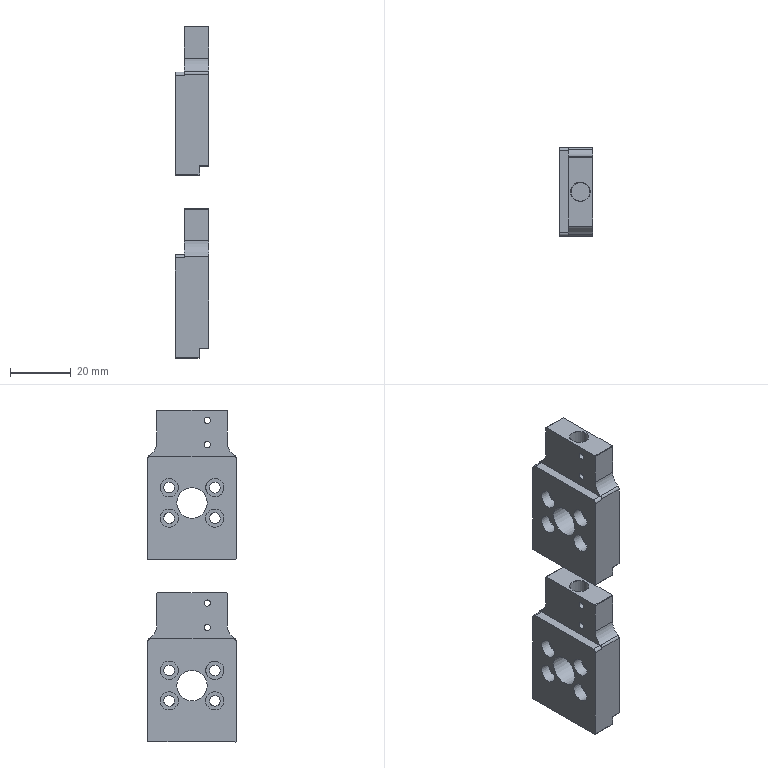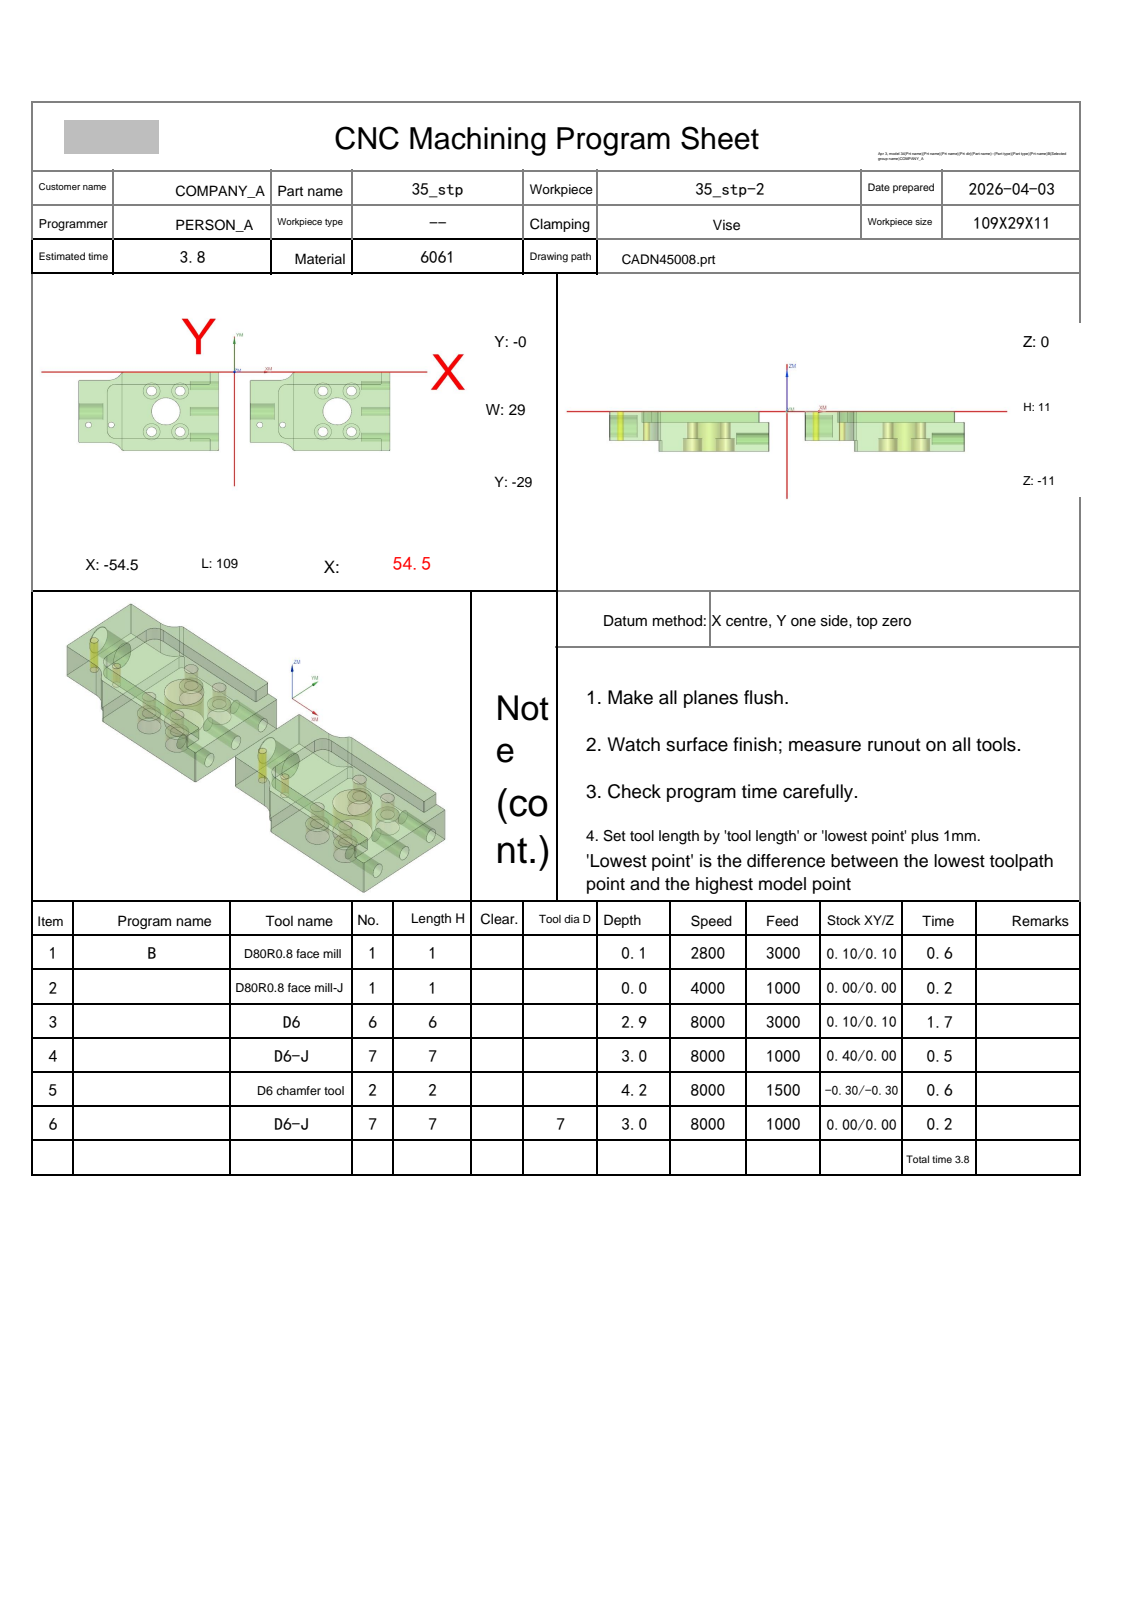NC program | NX | posted by the shop | part box 11 x 29 x 109 mm
Whole program:
%
O0001
(Machine time: 4.99 MIN)
(===Total Tool:4===)
(T1=D80R0.8 face mill D=80.  R=0.8  D-  H01 Z=-0.   )
(T6=D6      D=6.   R=0.   D-  H06 Z=-2.9  )
(T7=D6-J    D=6.   R=0.   D-  H07 Z=-3.   )
(T2=D6 chamfer tool   D=6.   R=0.   D-  H02 Z=-4.2  )
G80 G90 G17 G49 G40
G91 G28 Z0
M01
N1 T01 M06
(D80R0.8 face mill  D=80. R=0.8 H=01 ce=0.10 di=0.10)
G00 G90 G54 X-106.597 Y-14.5 M03 S2800
G43 H01 Z20.
M08
Z5.014
G01 Z3.014 F3000.
X-94.597
X94.597
X106.597
Z5.014
G00 X-106.597
Z4.529
G01 Z2.529
X-94.597
X94.597
X106.597
Z4.529
G00 X-106.597
Z4.043
G01 Z2.043
X-94.597
X94.597
X106.597
Z4.043
G00 X-106.597
Z3.557
G01 Z1.557
X-94.597
X94.597
X106.597
Z3.557
G00 Z20.
X-106.597
Z3.071
G01 Z1.071
X-94.597
X94.597
X106.597
Z3.071
G00 Z20.
X-106.597
Z2.586
G01 Z.586
X-94.597
X94.597
X106.597
Z2.586
G00 Z20.
X-106.597
Z2.1
G01 Z.1
X-94.597
X94.597
X106.597
Z2.1
G00 Z20.
G91 G28 Z0.0
M05
M09
G91 G28 Z0.0
M01
N2 T01 M06
(D80R0.8 face mill-J  D=80. R=0.8 H=01 ce=0.00 di=0.00)
G00 G90 G54 X-106.499 Y-14.5 M03 S4000
G43 H01 Z20.
M08
Z2.
G01 Z0.0 F1000.
X-94.499
X94.499
X106.499
Z2.
G00 Z20.
G91 G28 Z0.0
M05
M09
G91 G28 Z0.0
M01
N3 T06 M06
(D6  D=6. R=0. H=06 ce=0.10 di=0.10)
G00 G90 G54 X-2.569 Y-14.274 M03 S8000
G43 H06 Z13.5
M08
Z1.5
G02 X-2.569 Y-14.274 Z.611 I-2.691 J-.226 F3000.
X-2.569 Y-14.274 Z-.278 I-2.691 J-.226
X-2.56 Y-14.5 Z-.29 I-2.691 J-.226
G01 Y-29.818
X-4.682 Y-31.94
X-7.256
X-5.4 Y-30.084
Y-23.451
X-7.416 Y-21.435
X-41.435
Y-7.565
X-7.416
X-5.4 Y-5.549
Y1.084
X-7.256 Y2.94
X-2.56
Y-12.679
G02 X-2.827 Y-13.178 I-.6 J0.0
G01 X-6.793 Y-15.822
G03 X-7.06 Y-16.321 I.333 J-.499
G01 Y-16.336
G02 X-7.659 Y-16.935 I-.6 J.001
G01 X-36.336
G02 X-36.935 Y-16.336 I.001 J.6
G01 Y-12.664
G02 X-36.336 Y-12.065 I.6 J-.001
G01 X-7.659
G02 X-7.06 Y-12.664 I-.001 J-.6
G01 Y-14.5
Y-15.
X-4.06
Z1.21
G00 X-2.569 Y-14.274
G02 X-2.569 Y-14.274 Z.321 I-2.691 J-.226
X-2.569 Y-14.274 Z-.568 I-2.691 J-.226
X-2.56 Y-14.5 Z-.58 I-2.691 J-.226
G01 Y-29.818
X-4.682 Y-31.94
X-7.256
X-5.4 Y-30.084
Y-23.451
X-7.416 Y-21.435
X-41.435
Y-7.565
X-7.416
X-5.4 Y-5.549
Y1.084
X-7.256 Y2.94
X-2.56
Y-12.679
G02 X-2.827 Y-13.178 I-.6 J0.0
G01 X-6.793 Y-15.822
G03 X-7.06 Y-16.321 I.333 J-.499
G01 Y-16.336
G02 X-7.659 Y-16.935 I-.6 J.001
G01 X-36.336
G02 X-36.935 Y-16.336 I.001 J.6
G01 Y-12.664
G02 X-36.336 Y-12.065 I.6 J-.001
G01 X-7.659
G02 X-7.06 Y-12.664 I-.001 J-.6
G01 Y-14.5
Y-15.
X-4.06
Z.92
G00 X-2.569 Y-14.274
G02 X-2.569 Y-14.274 Z.031 I-2.691 J-.226
X-2.569 Y-14.274 Z-.858 I-2.691 J-.226
X-2.56 Y-14.5 Z-.87 I-2.691 J-.226
G01 Y-29.818
X-4.682 Y-31.94
X-7.256
X-5.4 Y-30.084
Y-23.451
X-7.416 Y-21.435
X-41.435
Y-7.565
X-7.416
X-5.4 Y-5.549
Y1.084
X-7.256 Y2.94
X-2.56
Y-12.679
G02 X-2.827 Y-13.178 I-.6 J0.0
G01 X-6.793 Y-15.822
G03 X-7.06 Y-16.321 I.333 J-.499
G01 Y-16.336
G02 X-7.659 Y-16.935 I-.6 J.001
G01 X-36.336
G02 X-36.935 Y-16.336 I.001 J.6
G01 Y-12.664
G02 X-36.336 Y-12.065 I.6 J-.001
G01 X-7.659
G02 X-7.06 Y-12.664 I-.001 J-.6
G01 Y-14.5
Y-15.
X-4.06
Z.63
G00 X-2.569 Y-14.274
G02 X-2.569 Y-14.274 Z-.259 I-2.691 J-.226
X-2.569 Y-14.274 Z-1.148 I-2.691 J-.226
X-2.56 Y-14.5 Z-1.16 I-2.691 J-.226
G01 Y-29.818
X-4.682 Y-31.94
X-7.256
X-5.4 Y-30.084
Y-23.451
X-7.416 Y-21.435
X-41.435
Y-7.565
X-7.416
X-5.4 Y-5.549
Y1.084
X-7.256 Y2.94
X-2.56
Y-12.679
G02 X-2.827 Y-13.178 I-.6 J0.0
G01 X-6.793 Y-15.822
G03 X-7.06 Y-16.321 I.333 J-.499
G01 Y-16.336
G02 X-7.659 Y-16.935 I-.6 J.001
G01 X-36.336
G02 X-36.935 Y-16.336 I.001 J.6
G01 Y-12.664
G02 X-36.336 Y-12.065 I.6 J-.001
G01 X-7.659
G02 X-7.06 Y-12.664 I-.001 J-.6
G01 Y-14.5
Y-15.
X-4.06
Z.34
G00 X-2.569 Y-14.274
G02 X-2.569 Y-14.274 Z-.549 I-2.691 J-.226
X-2.569 Y-14.274 Z-1.438 I-2.691 J-.226
X-2.56 Y-14.5 Z-1.45 I-2.691 J-.226
G01 Y-29.818
X-4.682 Y-31.94
X-7.256
X-5.4 Y-30.084
Y-23.451
X-7.416 Y-21.435
X-41.435
Y-7.565
X-7.416
X-5.4 Y-5.549
Y1.084
X-7.256 Y2.94
X-2.56
Y-12.679
G02 X-2.827 Y-13.178 I-.6 J0.0
G01 X-6.793 Y-15.822
G03 X-7.06 Y-16.321 I.333 J-.499
G01 Y-16.336
G02 X-7.659 Y-16.935 I-.6 J.001
G01 X-36.336
G02 X-36.935 Y-16.336 I.001 J.6
G01 Y-12.664
G02 X-36.336 Y-12.065 I.6 J-.001
G01 X-7.659
G02 X-7.06 Y-12.664 I-.001 J-.6
G01 Y-14.5
Y-15.
X-4.06
Z.05
G00 X-2.569 Y-14.274
G02 X-2.569 Y-14.274 Z-.839 I-2.691 J-.226
X-2.569 Y-14.274 Z-1.728 I-2.691 J-.226
X-2.56 Y-14.5 Z-1.74 I-2.691 J-.226
G01 Y-29.818
X-4.682 Y-31.94
X-7.256
X-5.4 Y-30.084
Y-23.451
X-7.416 Y-21.435
X-41.435
Y-7.565
X-7.416
X-5.4 Y-5.549
Y1.084
X-7.256 Y2.94
X-2.56
Y-12.679
G02 X-2.827 Y-13.178 I-.6 J0.0
G01 X-6.793 Y-15.822
G03 X-7.06 Y-16.321 I.333 J-.499
G01 Y-16.336
G02 X-7.659 Y-16.935 I-.6 J.001
G01 X-36.336
G02 X-36.935 Y-16.336 I.001 J.6
G01 Y-12.664
G02 X-36.336 Y-12.065 I.6 J-.001
G01 X-7.659
G02 X-7.06 Y-12.664 I-.001 J-.6
G01 Y-14.5
Y-15.
X-4.06
Z-.24
G00 X-2.569 Y-14.274
G02 X-2.569 Y-14.274 Z-1.129 I-2.691 J-.226
X-2.569 Y-14.274 Z-2.018 I-2.691 J-.226
X-2.56 Y-14.5 Z-2.03 I-2.691 J-.226
G01 Y-29.818
X-4.682 Y-31.94
X-7.256
X-5.4 Y-30.084
Y-23.451
X-7.416 Y-21.435
X-41.435
Y-7.565
X-7.416
X-5.4 Y-5.549
Y1.084
X-7.256 Y2.94
X-2.56
Y-12.679
G02 X-2.827 Y-13.178 I-.6 J0.0
G01 X-6.793 Y-15.822
G03 X-7.06 Y-16.321 I.333 J-.499
G01 Y-16.336
G02 X-7.659 Y-16.935 I-.6 J.001
G01 X-36.336
G02 X-36.935 Y-16.336 I.001 J.6
G01 Y-12.664
G02 X-36.336 Y-12.065 I.6 J-.001
G01 X-7.659
G02 X-7.06 Y-12.664 I-.001 J-.6
G01 Y-14.5
Y-15.
X-4.06
Z-.53
G00 X-2.569 Y-14.274
G02 X-2.569 Y-14.274 Z-1.419 I-2.691 J-.226
X-2.569 Y-14.274 Z-2.308 I-2.691 J-.226
X-2.56 Y-14.5 Z-2.32 I-2.691 J-.226
G01 Y-29.818
X-4.682 Y-31.94
X-7.256
X-5.4 Y-30.084
Y-23.451
X-7.416 Y-21.435
X-41.435
Y-7.565
X-7.416
X-5.4 Y-5.549
Y1.084
X-7.256 Y2.94
X-2.56
Y-12.679
G02 X-2.827 Y-13.178 I-.6 J0.0
G01 X-6.793 Y-15.822
G03 X-7.06 Y-16.321 I.333 J-.499
G01 Y-16.336
G02 X-7.659 Y-16.935 I-.6 J.001
G01 X-36.336
G02 X-36.935 Y-16.336 I.001 J.6
G01 Y-12.664
G02 X-36.336 Y-12.065 I.6 J-.001
G01 X-7.659
G02 X-7.06 Y-12.664 I-.001 J-.6
G01 Y-14.5
Y-15.
X-4.06
Z-.82
G00 X-2.569 Y-14.274
G02 X-2.569 Y-14.274 Z-1.709 I-2.691 J-.226
X-2.569 Y-14.274 Z-2.598 I-2.691 J-.226
X-2.56 Y-14.5 Z-2.61 I-2.691 J-.226
G01 Y-29.818
X-4.682 Y-31.94
X-7.256
X-5.4 Y-30.084
Y-23.451
X-7.416 Y-21.435
X-41.435
Y-7.565
X-7.416
X-5.4 Y-5.549
Y1.084
X-7.256 Y2.94
X-2.56
Y-12.679
G02 X-2.827 Y-13.178 I-.6 J0.0
G01 X-6.793 Y-15.822
G03 X-7.06 Y-16.321 I.333 J-.499
G01 Y-16.336
G02 X-7.659 Y-16.935 I-.6 J.001
G01 X-36.336
G02 X-36.935 Y-16.336 I.001 J.6
G01 Y-12.664
G02 X-36.336 Y-12.065 I.6 J-.001
G01 X-7.659
G02 X-7.06 Y-12.664 I-.001 J-.6
G01 Y-14.5
Y-15.
X-4.06
Z-1.11
G00 X-2.569 Y-14.274
G02 X-2.569 Y-14.274 Z-1.999 I-2.691 J-.226
X-2.569 Y-14.274 Z-2.888 I-2.691 J-.226
X-2.56 Y-14.5 Z-2.9 I-2.691 J-.226
G01 Y-29.818
X-4.682 Y-31.94
X-7.256
X-5.4 Y-30.084
Y-23.451
X-7.416 Y-21.435
X-41.435
Y-7.565
X-7.416
X-5.4 Y-5.549
Y1.084
X-7.256 Y2.94
X-2.56
Y-12.679
G02 X-2.827 Y-13.178 I-.6 J0.0
G01 X-6.793 Y-15.822
G03 X-7.06 Y-16.321 I.333 J-.499
G01 Y-16.336
G02 X-7.659 Y-16.935 I-.6 J.001
G01 X-36.336
G02 X-36.935 Y-16.336 I.001 J.6
G01 Y-12.664
G02 X-36.336 Y-12.065 I.6 J-.001
G01 X-7.659
G02 X-7.06 Y-12.664 I-.001 J-.6
G01 Y-14.5
Y-15.
X-4.06
Z-1.4
G00 Z13.5
X60.5 Y-14.5
Z1.21
G01 Z-.29
X57.44
Y-29.818
X55.318 Y-31.94
X52.744
X54.6 Y-30.084
Y-23.451
X52.584 Y-21.435
X18.565
Y-7.565
X52.584
X54.6 Y-5.549
Y1.084
X52.744 Y2.94
X57.44
Y-12.679
G02 X57.173 Y-13.178 I-.6 J0.0
G01 X53.207 Y-15.822
G03 X52.94 Y-16.321 I.333 J-.499
G01 Y-16.336
G02 X52.341 Y-16.935 I-.6 J.001
G01 X23.664
G02 X23.065 Y-16.336 I.001 J.6
G01 Y-12.664
G02 X23.664 Y-12.065 I.6 J-.001
G01 X52.341
G02 X52.94 Y-12.664 I-.001 J-.6
G01 Y-14.5
Y-15.
X60.5
Z1.21
G00 Y-14.5
Z.92
G01 Z-.58
X57.44
Y-29.818
X55.318 Y-31.94
X52.744
X54.6 Y-30.084
Y-23.451
X52.584 Y-21.435
X18.565
Y-7.565
X52.584
X54.6 Y-5.549
Y1.084
X52.744 Y2.94
X57.44
Y-12.679
G02 X57.173 Y-13.178 I-.6 J0.0
G01 X53.207 Y-15.822
G03 X52.94 Y-16.321 I.333 J-.499
G01 Y-16.336
G02 X52.341 Y-16.935 I-.6 J.001
G01 X23.664
G02 X23.065 Y-16.336 I.001 J.6
G01 Y-12.664
G02 X23.664 Y-12.065 I.6 J-.001
G01 X52.341
G02 X52.94 Y-12.664 I-.001 J-.6
G01 Y-14.5
Y-15.
X60.5
Z.92
G00 Y-14.5
Z.63
G01 Z-.87
X57.44
Y-29.818
X55.318 Y-31.94
X52.744
X54.6 Y-30.084
Y-23.451
X52.584 Y-21.435
X18.565
Y-7.565
X52.584
X54.6 Y-5.549
Y1.084
X52.744 Y2.94
X57.44
Y-12.679
G02 X57.173 Y-13.178 I-.6 J0.0
G01 X53.207 Y-15.822
G03 X52.94 Y-16.321 I.333 J-.499
G01 Y-16.336
G02 X52.341 Y-16.935 I-.6 J.001
G01 X23.664
G02 X23.065 Y-16.336 I.001 J.6
G01 Y-12.664
G02 X23.664 Y-12.065 I.6 J-.001
G01 X52.341
G02 X52.94 Y-12.664 I-.001 J-.6
G01 Y-14.5
Y-15.
X60.5
Z.63
G00 Y-14.5
Z.34
G01 Z-1.16
X57.44
Y-29.818
X55.318 Y-31.94
X52.744
X54.6 Y-30.084
Y-23.451
X52.584 Y-21.435
X18.565
Y-7.565
X52.584
X54.6 Y-5.549
Y1.084
X52.744 Y2.94
X57.44
Y-12.679
G02 X57.173 Y-13.178 I-.6 J0.0
G01 X53.207 Y-15.822
G03 X52.94 Y-16.321 I.333 J-.499
G01 Y-16.336
G02 X52.341 Y-16.935 I-.6 J.001
G01 X23.664
G02 X23.065 Y-16.336 I.001 J.6
G01 Y-12.664
G02 X23.664 Y-12.065 I.6 J-.001
G01 X52.341
G02 X52.94 Y-12.664 I-.001 J-.6
G01 Y-14.5
Y-15.
X60.5
Z.34
G00 Y-14.5
Z.05
G01 Z-1.45
X57.44
Y-29.818
X55.318 Y-31.94
X52.744
X54.6 Y-30.084
Y-23.451
X52.584 Y-21.435
X18.565
Y-7.565
X52.584
X54.6 Y-5.549
Y1.084
X52.744 Y2.94
X57.44
Y-12.679
G02 X57.173 Y-13.178 I-.6 J0.0
G01 X53.207 Y-15.822
G03 X52.94 Y-16.321 I.333 J-.499
G01 Y-16.336
G02 X52.341 Y-16.935 I-.6 J.001
G01 X23.664
G02 X23.065 Y-16.336 I.001 J.6
G01 Y-12.664
G02 X23.664 Y-12.065 I.6 J-.001
G01 X52.341
G02 X52.94 Y-12.664 I-.001 J-.6
G01 Y-14.5
Y-15.
X60.5
Z.05
G00 Y-14.5
Z-.24
G01 Z-1.74
X57.44
Y-29.818
X55.318 Y-31.94
X52.744
X54.6 Y-30.084
Y-23.451
X52.584 Y-21.435
X18.565
Y-7.565
X52.584
X54.6 Y-5.549
Y1.084
X52.744 Y2.94
X57.44
Y-12.679
G02 X57.173 Y-13.178 I-.6 J0.0
G01 X53.207 Y-15.822
G03 X52.94 Y-16.321 I.333 J-.499
G01 Y-16.336
G02 X52.341 Y-16.935 I-.6 J.001
G01 X23.664
G02 X23.065 Y-16.336 I.001 J.6
G01 Y-12.664
G02 X23.664 Y-12.065 I.6 J-.001
G01 X52.341
G02 X52.94 Y-12.664 I-.001 J-.6
G01 Y-14.5
Y-15.
X60.5
Z-.24
G00 Y-14.5
Z-.53
G01 Z-2.03
X57.44
Y-29.818
X55.318 Y-31.94
X52.744
X54.6 Y-30.084
Y-23.451
X52.584 Y-21.435
X18.565
Y-7.565
X52.584
X54.6 Y-5.549
Y1.084
X52.744 Y2.94
X57.44
Y-12.679
G02 X57.173 Y-13.178 I-.6 J0.0
G01 X53.207 Y-15.822
G03 X52.94 Y-16.321 I.333 J-.499
G01 Y-16.336
G02 X52.341 Y-16.935 I-.6 J.001
G01 X23.664
G02 X23.065 Y-16.336 I.001 J.6
G01 Y-12.664
G02 X23.664 Y-12.065 I.6 J-.001
G01 X52.341
G02 X52.94 Y-12.664 I-.001 J-.6
G01 Y-14.5
Y-15.
X60.5
Z-.53
G00 Y-14.5
Z-.82
G01 Z-2.32
X57.44
Y-29.818
X55.318 Y-31.94
X52.744
X54.6 Y-30.084
Y-23.451
X52.584 Y-21.435
X18.565
Y-7.565
X52.584
X54.6 Y-5.549
Y1.084
X52.744 Y2.94
X57.44
Y-12.679
G02 X57.173 Y-13.178 I-.6 J0.0
G01 X53.207 Y-15.822
G03 X52.94 Y-16.321 I.333 J-.499
G01 Y-16.336
G02 X52.341 Y-16.935 I-.6 J.001
G01 X23.664
G02 X23.065 Y-16.336 I.001 J.6
G01 Y-12.664
G02 X23.664 Y-12.065 I.6 J-.001
G01 X52.341
G02 X52.94 Y-12.664 I-.001 J-.6
G01 Y-14.5
Y-15.
X60.5
Z-.82
G00 Y-14.5
Z-1.11
G01 Z-2.61
X57.44
Y-29.818
X55.318 Y-31.94
X52.744
X54.6 Y-30.084
Y-23.451
X52.584 Y-21.435
X18.565
Y-7.565
X52.584
X54.6 Y-5.549
Y1.084
X52.744 Y2.94
X57.44
Y-12.679
G02 X57.173 Y-13.178 I-.6 J0.0
G01 X53.207 Y-15.822
G03 X52.94 Y-16.321 I.333 J-.499
G01 Y-16.336
G02 X52.341 Y-16.935 I-.6 J.001
G01 X23.664
G02 X23.065 Y-16.336 I.001 J.6
G01 Y-12.664
G02 X23.664 Y-12.065 I.6 J-.001
G01 X52.341
G02 X52.94 Y-12.664 I-.001 J-.6
G01 Y-14.5
Y-15.
X60.5
Z-1.11
G00 Y-14.5
Z-1.4
G01 Z-2.9
X57.44
Y-29.818
X55.318 Y-31.94
X52.744
X54.6 Y-30.084
Y-23.451
X52.584 Y-21.435
X18.565
Y-7.565
X52.584
X54.6 Y-5.549
Y1.084
X52.744 Y2.94
X57.44
Y-12.679
G02 X57.173 Y-13.178 I-.6 J0.0
G01 X53.207 Y-15.822
G03 X52.94 Y-16.321 I.333 J-.499
G01 Y-16.336
G02 X52.341 Y-16.935 I-.6 J.001
G01 X23.664
G02 X23.065 Y-16.336 I.001 J.6
G01 Y-12.664
G02 X23.664 Y-12.065 I.6 J-.001
G01 X52.341
G02 X52.94 Y-12.664 I-.001 J-.6
G01 Y-14.5
Y-15.
X60.5
Z-1.4
G00 Z13.5
G91 G28 Z0.0
M05
M09
G91 G28 Z0.0
M01
N4 T07 M06
(D6-J  D=6. R=0. H=07 ce=0.40 di=0.00)
G00 G90 G54 X-1.3 Y-13.3 M03 S8000
G43 H07 Z13.5
M08
Z-1.5
G01 Z-3. F1000.
X-3.7
G03 X-4.9 Y-14.5 I0.0 J-1.2
G01 Y-23.238
X-5.02 Y-23.357
X-5.104 Y-23.322
X-7.292 Y-21.135
X-40.537
G02 X-41.135 Y-20.537 I.002 J.6
G01 Y-8.464
G02 X-40.537 Y-7.865 I.6 J-.002
G01 X-7.292
X-5.104 Y-5.678
X-5.02 Y-5.643
X-4.9 Y-5.762
Y-15.633
G02 X-5.226 Y-16.167 I-.6 J0.0
G01 X-7.644 Y-17.406
G03 X-7.935 Y-17.737 I.274 J-.534
G02 X-8.498 Y-18.135 I-.565 J.202
G01 X-37.537
G02 X-38.135 Y-17.537 I.002 J.6
G01 Y-11.463
G02 X-37.537 Y-10.865 I.6 J-.002
G01 X-8.498
G02 X-7.9 Y-11.463 I-.002 J-.6
G01 Y-15.421
G02 X-8.38 Y-15.901 I-.48 J0.0
G01 X-8.469 Y-15.892
X-12.416 Y-15.145
X-12.47 Y-15.128
X-12.527 Y-15.135
X-34.537
G02 X-35.135 Y-14.537 I.002 J.6
G01 Y-14.463
G02 X-34.537 Y-13.865 I.6 J-.002
G01 X-11.498
G02 X-10.9 Y-14.463 I-.002 J-.6
G01 Y-14.537
G02 X-11.037 Y-14.916 I-.6 J.002
X-11.498 Y-15.135 I-.463 J.381
G01 X-11.971
G03 X-13.171 Y-16.335 I0.0 J-1.2
G01 Z-1.5
G00 Z13.5
X58.7 Y-13.3
Z-1.5
G01 Z-3.
X56.3
G03 X55.1 Y-14.5 I0.0 J-1.2
G01 Y-23.238
X54.98 Y-23.357
X54.896 Y-23.322
X52.708 Y-21.135
X19.464
G02 X18.865 Y-20.536 I.001 J.6
G01 Y-8.464
G02 X19.464 Y-7.865 I.6 J-.001
G01 X52.708
X54.896 Y-5.678
X54.98 Y-5.643
X55.1 Y-5.762
Y-17.5
G02 X54.5 Y-18.1 I-.6 J0.0
G01 X54.359 Y-18.083
X52.61 Y-17.66
X52.469 Y-17.643
G03 X51.985 Y-17.889 I0.0 J-.6
G02 X51.502 Y-18.135 I-.485 J.354
G01 X22.463
G02 X21.865 Y-17.537 I.002 J.6
G01 Y-11.463
G02 X22.463 Y-10.865 I.6 J-.002
G01 X51.502
G02 X52.1 Y-11.463 I-.002 J-.6
G01 Y-15.421
G02 X51.62 Y-15.901 I-.48 J0.0
G01 X51.531 Y-15.892
X47.584 Y-15.145
X47.53 Y-15.128
X47.473 Y-15.135
X25.463
G02 X24.865 Y-14.537 I.002 J.6
G01 Y-14.463
G02 X25.463 Y-13.865 I.6 J-.002
G01 X48.502
G02 X49.1 Y-14.463 I-.002 J-.6
G01 Y-14.537
G02 X48.963 Y-14.916 I-.6 J.002
X48.502 Y-15.135 I-.463 J.381
G01 X48.029
G03 X46.829 Y-16.335 I0.0 J-1.2
G01 Z-1.5
G00 Z13.5
G91 G28 Z0.0
M05
M09
G91 G28 Z0.0
M01
N5 T02 M06
(D6 chamfer tool  D=6. R=0. H=02 ce=0.00 di=0.00)
G00 G90 G54 X-51.1 Y-19.5 M03 S8000
G43 H02 Z20.
M08
G98 G81 X-51.1 Y-19.5 Z-1.35 R3. F1000.
X8.9
G80
G00 Z20.
G00 G90 X-22.7 Y-17.5 M03 S8000
Z20.
Z-3.5
G01 Z-4. F1200.
G03 X-19.7 Y-14.5 I0.0 J3.
X-24. Y-10.2 I-4.3 J0.0
X-28.3 Y-14.5 I0.0 J-4.3
X-24. Y-18.8 I4.3 J0.0
X-19.7 Y-14.5 I0.0 J4.3
X-22.7 Y-11.5 I-3. J0.0
G01 Z-3.5
G00 Z20.
X37.3 Y-17.5
Z-3.5
G01 Z-4.
G03 X40.3 Y-14.5 I0.0 J3.
X36. Y-10.2 I-4.3 J0.0
X31.7 Y-14.5 I0.0 J-4.3
X36. Y-18.8 I4.3 J0.0
X40.3 Y-14.5 I0.0 J4.3
X37.3 Y-11.5 I-3. J0.0
G01 Z-3.5
G00 Z20.
G00 G90 X-25.486 Y-23.308 M03 S6500
Z20.
Z.172
G01 Z-1.199 F1500.
G03 X-25.2 Y-23.508 I1.286 J1.532
G01 X-25.154 Y-23.538
X-25.1 Y-23.535
X-8.7
X-8.441 Y-23.569
X-8.2 Y-23.669
X-7.993 Y-23.828
X-7.793 Y-24.028
X-7.634 Y-24.235
X-7.534 Y-24.476
X-7.5 Y-24.735
Y-28.8
X-7.534 Y-29.059
X-7.634 Y-29.3
X-7.793 Y-29.507
X-7.993 Y-29.707
X-8.2 Y-29.866
X-8.441 Y-29.966
X-8.7 Y-30.
X-38.736
G02 X-40.468 Y-29. I0.0 J2.
G03 X-43.933 Y-27. I-3.464 J-2.
G01 X-54.3
X-54.559 Y-26.966
X-54.8 Y-26.866
X-55.007 Y-26.707
X-55.207 Y-26.507
X-55.366 Y-26.3
X-55.466 Y-26.059
X-55.5 Y-25.8
Y-3.2
X-55.466 Y-2.941
X-55.366 Y-2.7
X-55.207 Y-2.493
X-55.007 Y-2.293
X-54.8 Y-2.134
X-54.559 Y-2.034
X-54.3 Y-2.
X-43.933
G03 X-40.468 Y0.0 I0.0 J4.
G02 X-38.736 Y1. I1.732 J-1.
G01 X-8.7
X-8.441 Y.966
X-8.2 Y.866
X-7.993 Y.707
X-7.793 Y.507
X-7.634 Y.3
X-7.534 Y.059
X-7.5 Y-.2
Y-4.265
X-7.534 Y-4.524
X-7.634 Y-4.765
X-7.793 Y-4.972
X-7.993 Y-5.172
X-8.2 Y-5.331
X-8.441 Y-5.431
X-8.7 Y-5.465
X-41.5
G03 X-43.535 Y-7.5 I0.0 J-2.035
G01 Y-21.5
G03 X-41.5 Y-23.535 I2.035 J0.0
G01 X-25.1
X-25.046 Y-23.538
X-25. Y-23.508
G03 X-24.714 Y-23.308 I-1. J1.732
G01 Z.172
G00 Z10.
X35.286 Y-5.692
Z.172
G01 Z-1.199
G03 X35. Y-5.492 I-1.286 J-1.532
G01 X34.954 Y-5.462
X34.9 Y-5.465
X18.5
G03 X16.465 Y-7.5 I0.0 J-2.035
G01 Y-21.5
G03 X18.5 Y-23.535 I2.035 J0.0
G01 X51.3
X51.559 Y-23.569
X51.8 Y-23.669
X52.007 Y-23.828
X52.207 Y-24.028
X52.366 Y-24.235
X52.466 Y-24.476
X52.5 Y-24.735
Y-28.8
X52.466 Y-29.059
X52.366 Y-29.3
X52.207 Y-29.507
X52.007 Y-29.707
X51.8 Y-29.866
X51.559 Y-29.966
X51.3 Y-30.
X21.264
G02 X19.532 Y-29. I0.0 J2.
G03 X16.067 Y-27. I-3.464 J-2.
G01 X5.7
X5.441 Y-26.966
X5.2 Y-26.866
X4.993 Y-26.707
X4.793 Y-26.507
X4.634 Y-26.3
X4.534 Y-26.059
X4.5 Y-25.8
Y-3.2
X4.534 Y-2.941
X4.634 Y-2.7
X4.793 Y-2.493
X4.993 Y-2.293
X5.2 Y-2.134
X5.441 Y-2.034
X5.7 Y-2.
X16.067
G03 X19.532 Y0.0 I0.0 J4.
G02 X21.264 Y1. I1.732 J-1.
G01 X51.3
X51.559 Y.966
X51.8 Y.866
X52.007 Y.707
X52.207 Y.507
X52.366 Y.3
X52.466 Y.059
X52.5 Y-.2
Y-4.265
X52.466 Y-4.524
X52.366 Y-4.765
X52.207 Y-4.972
X52.007 Y-5.172
X51.8 Y-5.331
X51.559 Y-5.431
X51.3 Y-5.465
X34.9
X34.846 Y-5.462
X34.8 Y-5.492
G03 X34.514 Y-5.692 I1. J-1.732
G01 Z.172
G00 Z10.
X-5.576 Y1.102
Z-1.802
G01 Z-4.199
X-5.534 Y1.045
X-5.474 Y1.007
X-5.459 Y.988
X-5.435 Y.991
X-5.241 Y.966
G02 X-4.5 Y0.0 I-.259 J-.966
G01 Y-1.788
Y-3.575
Y-7.15
Y-14.3
Y-19.663
Y-23.238
Y-25.025
Y-28.6
X-4.534 Y-28.859
X-4.597 Y-29.01
Z-.199
G00 Z10.
X-19.176 Y-7.674
Z-1.81
G01 Z-4.199
X-19.129 Y-7.726
X-19.111 Y-7.735
X-19.056 Y-7.748
X-18.889 Y-7.735
X-18.86 Y-7.725
X-18.779 Y-7.659
Z-1.795
G00 Z-.449
X-29.176 Y-7.674
Z-1.81
G01 Z-4.199
X-29.129 Y-7.726
X-29.111 Y-7.735
X-29.056 Y-7.748
X-28.889 Y-7.735
X-28.86 Y-7.725
X-28.779 Y-7.659
Z-1.795
G00 Z-.449
X-20.201 Y-14.9
Z-2.775
G01 Z-4.199
G03 X-20.02 Y-14.602 I-1.613 J1.183
G01 X-19.994 Y-14.554
X-20. Y-14.5
G03 X-24. Y-10.5 I-4. J0.0
X-28. Y-14.5 I0.0 J-4.
X-24. Y-18.5 I4. J0.0
X-20. Y-14.5 I0.0 J4.
G01 X-19.994 Y-14.446
X-20.02 Y-14.398
G03 X-20.201 Y-14.1 I-1.794 J-.885
G01 Z-2.775
G00 Z-.449
X-28.779 Y-21.341
Z-1.795
G01 Z-4.199
X-28.86 Y-21.275
X-28.889 Y-21.265
X-29.056 Y-21.252
X-29.111 Y-21.265
X-29.129 Y-21.274
X-29.176 Y-21.326
Z-1.81
G00 Z-.449
X-18.779 Y-21.341
Z-1.795
G01 Z-4.199
X-18.86 Y-21.275
X-18.889 Y-21.265
X-19.056 Y-21.252
X-19.111 Y-21.265
X-19.129 Y-21.274
X-19.176 Y-21.326
Z-1.81
G00 Z10.
X54.424 Y1.102
Z-1.802
G01 Z-4.199
X54.466 Y1.045
X54.526 Y1.007
X54.541 Y.988
X54.565 Y.991
X54.759 Y.966
G02 X55.5 Y0.0 I-.259 J-.966
G01 Y-1.788
Y-3.575
Y-7.15
Y-14.3
Y-19.663
Y-23.238
Y-25.025
Y-28.6
X55.466 Y-28.859
X55.403 Y-29.01
Z-.199
G00 Z10.
X40.824 Y-7.674
Z-1.81
G01 Z-4.199
X40.871 Y-7.726
X40.889 Y-7.735
X40.944 Y-7.748
X41.111 Y-7.735
X41.14 Y-7.725
X41.221 Y-7.659
Z-1.795
G00 Z-.449
X30.824 Y-7.674
Z-1.81
G01 Z-4.199
X30.871 Y-7.726
X30.889 Y-7.735
X30.944 Y-7.748
X31.111 Y-7.735
X31.14 Y-7.725
X31.221 Y-7.659
Z-1.795
G00 Z-.449
X39.799 Y-14.9
Z-2.775
G01 Z-4.199
G03 X39.98 Y-14.602 I-1.613 J1.183
G01 X40.006 Y-14.554
X40. Y-14.5
G03 X36. Y-10.5 I-4. J0.0
X32. Y-14.5 I0.0 J-4.
X36. Y-18.5 I4. J0.0
X40. Y-14.5 I0.0 J4.
G01 X40.006 Y-14.446
X39.98 Y-14.398
G03 X39.799 Y-14.1 I-1.794 J-.885
G01 Z-2.775
G00 Z-.449
X41.221 Y-21.341
Z-1.795
G01 Z-4.199
X41.14 Y-21.275
X41.111 Y-21.265
X40.944 Y-21.252
X40.889 Y-21.265
X40.871 Y-21.274
X40.824 Y-21.326
Z-1.81
G00 Z-.449
X31.221 Y-21.341
Z-1.795
G01 Z-4.199
X31.14 Y-21.275
X31.111 Y-21.265
X30.944 Y-21.252
X30.889 Y-21.265
X30.871 Y-21.274
X30.824 Y-21.326
Z-1.81
G00 Z20.
G91 G28 Z0.0
M05
M09
G91 G28 Z0.0
M01
N6 T07 M06
(D6-J  D=6. R=0. H=07 ce=0.00 di=0.00)
G00 G90 G54 X-7.698 Y4.391 M03 S8000
G43 H07 Z13.5
M08
Z-2.
G01 Z-3. F1000.
G41 D07
X-7.756 Y4.2
G03 X-7.809 Y3.849 I1.147 J-.351
X-7.457 Y3. I1.2 J0.0
G01 X-5.5 Y1.043
Y-5.508
X-7.457 Y-7.465
X-41.5
X-41.519 Y-7.467
X-41.533 Y-7.481
X-41.535 Y-7.5
Y-21.5
X-41.533 Y-21.519
X-41.519 Y-21.533
X-41.5 Y-21.535
X-7.457
X-5.5 Y-23.492
Y-30.043
X-7.457 Y-32.
G03 X-7.809 Y-32.849 I.849 J-.849
X-7.756 Y-33.2 I1.2 J0.0
G01 G40 X-7.698 Y-33.391
Z-2.
G00 Z13.5
X52.302 Y4.391
Z-2.
G01 Z-3.
G41 D07
X52.244 Y4.2
G03 X52.191 Y3.849 I1.147 J-.351
X52.543 Y3. I1.2 J0.0
G01 X54.5 Y1.043
Y-5.508
X52.543 Y-7.465
X18.5
X18.481 Y-7.467
X18.467 Y-7.481
X18.465 Y-7.5
Y-21.5
X18.467 Y-21.519
X18.481 Y-21.533
X18.5 Y-21.535
X52.543
X54.5 Y-23.492
Y-30.043
X52.543 Y-32.
G03 X52.191 Y-32.849 I.849 J-.849
X52.244 Y-33.2 I1.2 J0.0
G01 G40 X52.302 Y-33.391
Z-2.
G00 Z13.5
M05
M09
G91 G28 Z0.0
G91 G28 Y0.0
M30
%